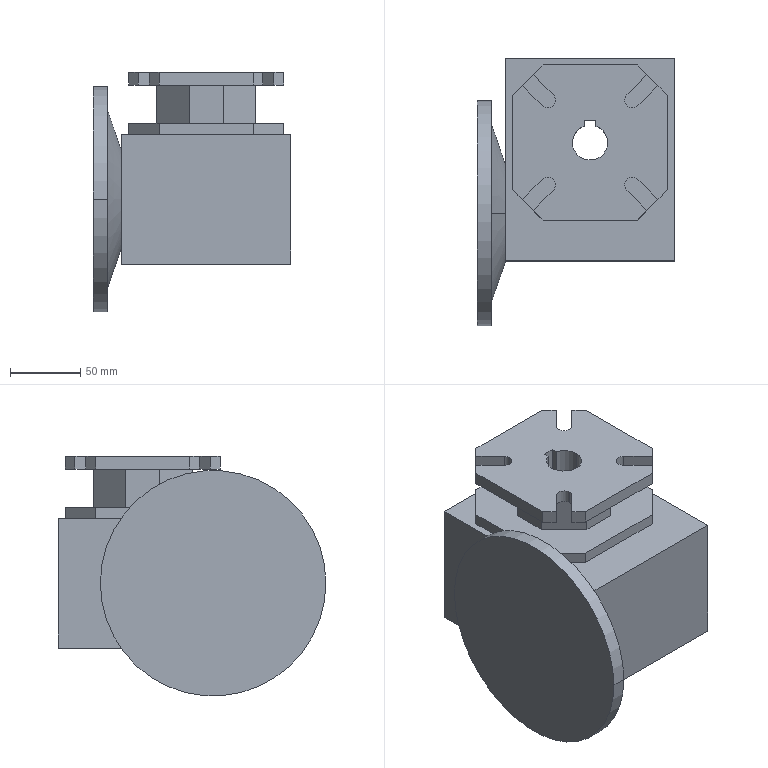Part | 1 solid | 63 faces | box 140 x 190 x 170 mm | volume 2080548 mm3 | plane 50 | cylinder 11 | cone 2 | commonest cylinder face diameters 11 x6 25 x3 160 x2